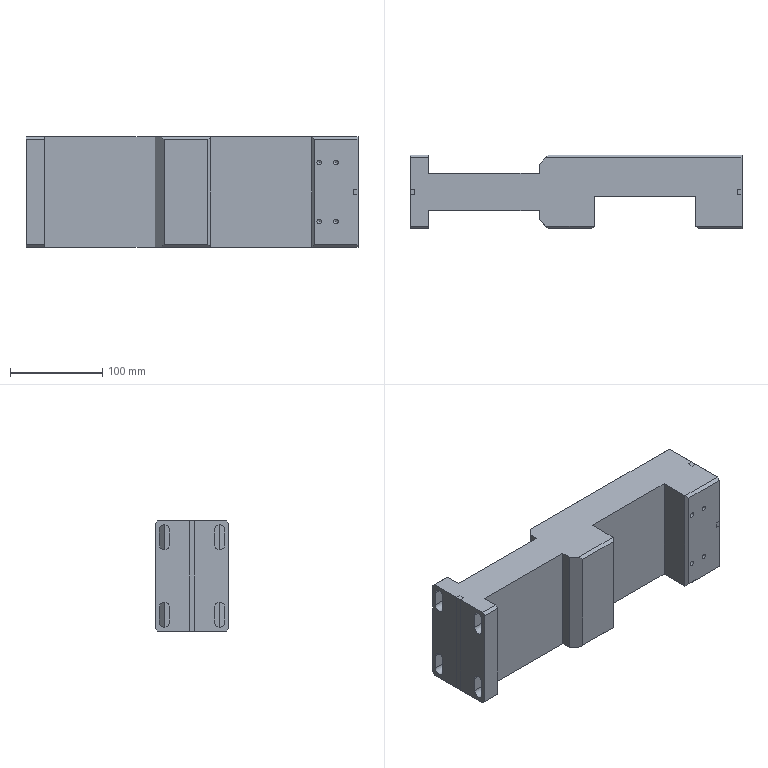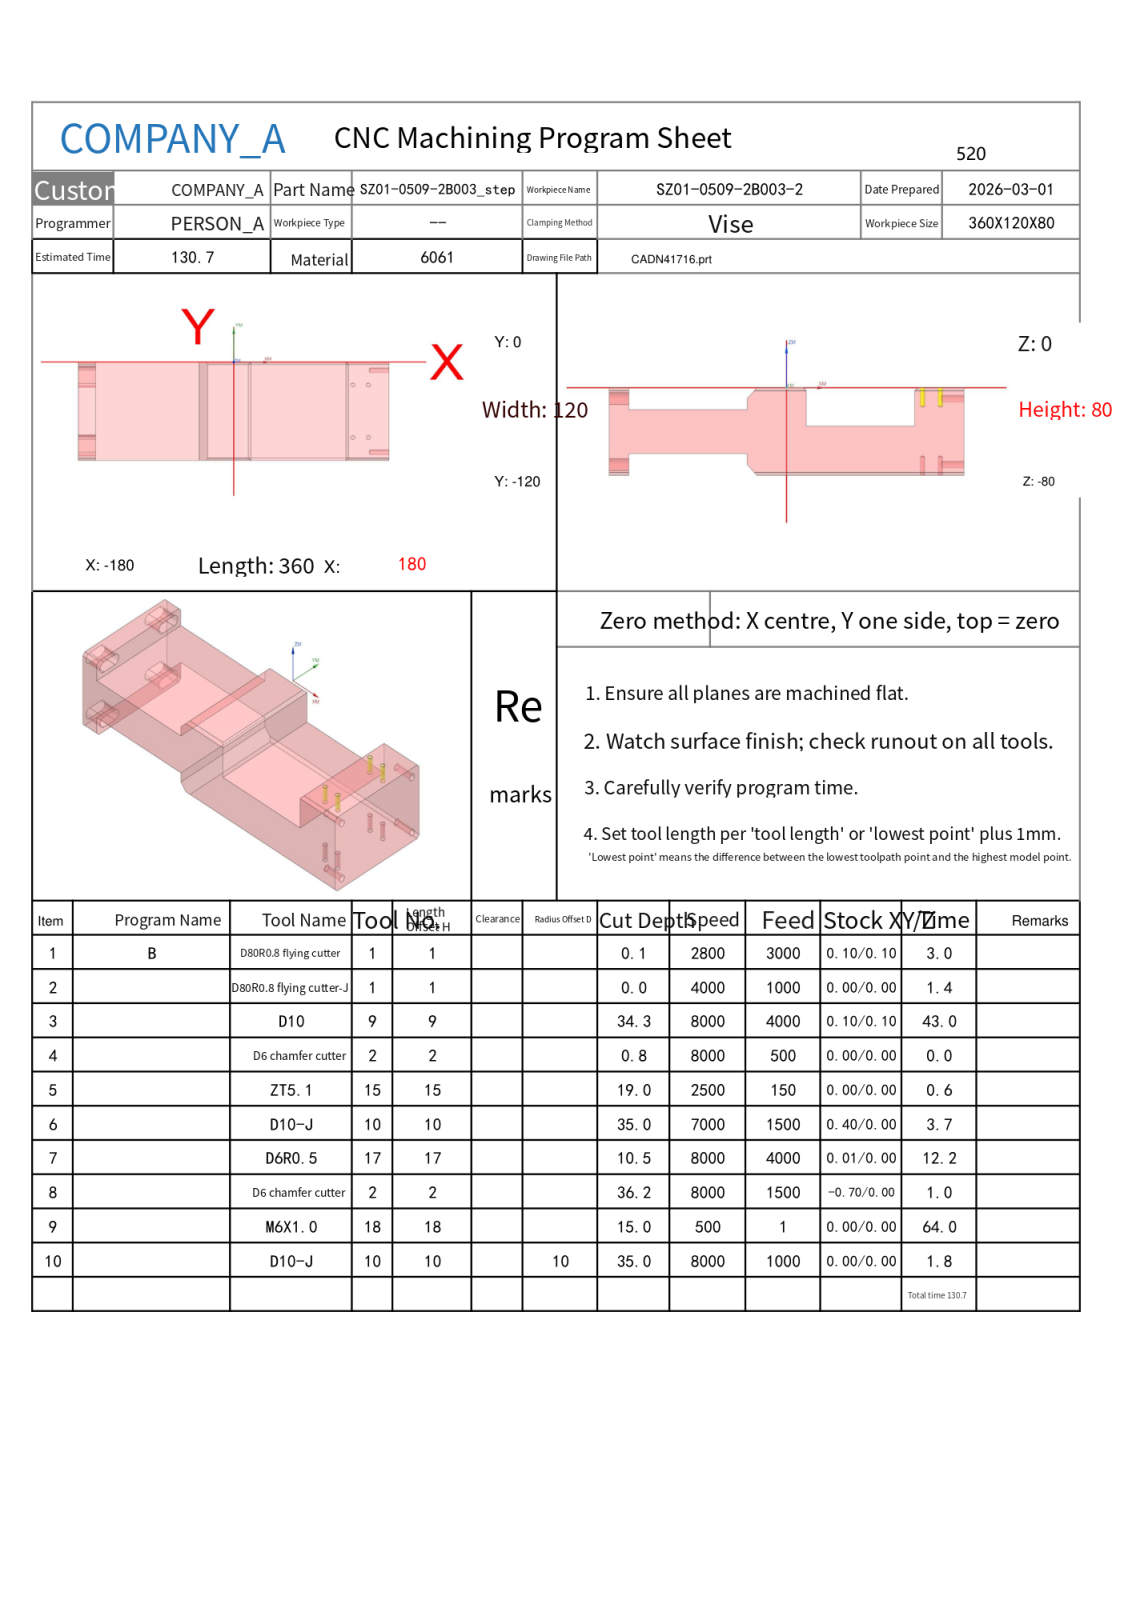NC program | NX | posted by the shop | part box 360 x 80 x 120 mm
Lines 151 to 1270 of 12457:
N3 T09 M06
(D10  D=10. R=0. H=09 ce=0.10 di=0.10)
G00 G90 G54 X-85.526 Y-134.5 M03 S8000
G43 H09 Z14.5
M08
Z.514
G01 Z-.686 F4000.
Y-127.081
G03 X-92.526 Y-120.081 I-7. J0.0
G01 X-153.947 Y-120.08
X-154.822
G02 X-155.408 Y-122.316 I-5.247 J.18
X-155.832 Y-123. I-4.662 J2.416
G01 X-156.212
G02 X-160. Y-124.228 I-3.808 J5.293
G01 X-179.919
Y-123.
X-180.
Y-124.228
Y-123.
X-180.08
X-180.079 Y-122.828
X-180.001
X-180.
X-179.999
X-179.919
X-178.519
X-160.
G03 X-154.903 Y-117.896 I-.021 J5.121
G01 X-154.866 Y-117.691
X-154.82 Y-116.969
Y-116.774
Y-116.578
Y-116.189
Y-115.297
Y-114.405
X-154.821 Y-113.513
Y-58.662
Y-3.812
X-154.822 Y-2.914
X-154.867 Y-2.301
X-154.903 Y-2.104
G03 X-160. Y2.828 I-5.117 J-.189
G01 X-178.52
X-179.92
X-179.999
X-180.
X-180.001
X-180.08
Y3.
X-180.
Y4.228
Y3.
X-179.92
Y4.228
X-159.994
G02 X-156.213 Y3. I-.026 J-6.521
G01 X-155.849
G02 X-155.456 Y2.363 I-4.505 J-3.224
X-154.823 Y.08 I-4.899 J-2.587
G01 X-44.966
X-38.144
X-38.087 Y.66
G02 X-37.123 Y3. I5.19 J-.768
G01 X-34.549
G02 X-30.757 Y4.228 I3.792 J-5.243
G01 X17.757
G02 X21.549 Y3. I0.0 J-6.471
G01 X24.114
G02 X25.148 Y.08 I-4.246 J-3.147
G01 X25.932
X124.296
X124.852
G02 X125.852 Y3. I5.632 J-.298
G01 X128.451
G02 X132.243 Y4.228 I3.792 J-5.243
G01 X179.92
Y3.
X180.
Y4.228
Y3.
X180.08
Y2.828
X180.001
X180.
X179.999
X179.92
X178.52
X132.243
G03 X127.172 Y-2.243 I0.0 J-5.071
G01 Y-117.757
G03 X132.243 Y-122.828 I5.071 J0.0
G01 X178.519
X179.919
X180.079
Y-123.
X179.919
Y-124.228
X132.243
G02 X128.452 Y-123. I0.0 J6.471
G01 X125.892
G02 X124.852 Y-120.08 I4.35 J3.193
G01 X28.427
G02 X27.486 Y-119.417 I.001 J1.
G01 X25.406 Y-113.592
G03 X24.846 Y-113.005 I-.941 J-.337
G02 X24.228 Y-112.085 I.381 J.924
G01 Y-7.915
G02 X25.223 Y-6.92 I1. J-.005
G01 X25.933
X119.177
G02 X120.172 Y-7.915 I-.005 J-1.
G01 Y-112.085
G02 X119.177 Y-113.08 I-1. J.005
G01 X28.721
G02 X28.022 Y-112.38 I.001 J.7
X28.064 Y-112.142 I.7 J0.0
G01 X31.168 Y-103.596
G03 X31.228 Y-103.256 I-.94 J.341
G01 Y-14.915
G02 X32.223 Y-13.92 I1. J-.005
G01 X112.177
G02 X113.172 Y-14.915 I-.005 J-1.
G01 Y-105.085
G02 X112.177 Y-106.08 I-1. J.005
G01 X34.923
G02 X34.323 Y-105.48 I0.0 J.6
X34.373 Y-105.241 I.6 J0.0
G01 X38.145 Y-96.562
G03 X38.228 Y-96.164 I-.917 J.398
G01 Y-21.915
G02 X39.222 Y-20.92 I1. J-.005
G01 X105.178
G02 X106.172 Y-21.915 I-.005 J-1.
G01 Y-98.085
G02 X105.178 Y-99.08 I-1. J.005
G01 X41.868
G02 X41.268 Y-98.48 I0.0 J.6
X41.319 Y-98.239 I.6 J0.0
G01 X45.143 Y-89.558
G03 X45.228 Y-89.156 I-.915 J.403
G01 Y-28.915
G02 X46.222 Y-27.92 I1. J-.005
G01 X98.178
G02 X99.172 Y-28.915 I-.005 J-1.
G01 Y-91.085
G02 X98.178 Y-92.08 I-1. J.005
G01 X48.863
G02 X48.263 Y-91.48 I0.0 J.6
X48.314 Y-91.238 I.6 J0.0
G01 X52.143 Y-82.558
G03 X52.228 Y-82.155 I-.915 J.403
G01 Y-35.914
G02 X53.222 Y-34.92 I1. J-.006
G01 X91.178
G02 X92.172 Y-35.914 I-.006 J-1.
G01 Y-84.086
G02 X91.178 Y-85.08 I-1. J.006
G01 X55.862
G02 X55.263 Y-84.48 I0.0 J.6
X55.314 Y-84.238 I.6 J0.0
G01 X59.143 Y-75.558
G03 X59.228 Y-75.155 I-.915 J.403
G01 Y-42.914
G02 X60.222 Y-41.92 I1. J-.006
G01 X84.178
G02 X85.172 Y-42.914 I-.006 J-1.
G01 Y-77.086
G02 X84.178 Y-78.08 I-1. J.006
G01 X62.862
G02 X62.263 Y-77.48 I0.0 J.6
X62.314 Y-77.238 I.6 J0.0
G01 X66.143 Y-68.558
G03 X66.228 Y-68.155 I-.915 J.403
G01 Y-49.914
G02 X67.222 Y-48.92 I1. J-.006
G01 X77.178
G02 X78.172 Y-49.914 I-.006 J-1.
G01 Y-70.086
G02 X77.178 Y-71.08 I-1. J.006
G01 X69.836
G02 X69.137 Y-70.38 I0.0 J.7
G01 X69.157 Y-70.212
X70.698 Y-63.983
G03 X70.728 Y-63.744 I-.971 J.24
G01 Y-54.414
G02 X71.722 Y-53.42 I1. J-.006
G01 X72.678
G02 X73.672 Y-54.414 I-.006 J-1.
G01 Y-65.586
G02 X72.854 Y-66.563 I-1. J.006
G03 X72.472 Y-66.721 I.182 J-.983
G01 X66.597 Y-70.735
X66.455 Y-70.853
X59.521 Y-77.787
X52.521 Y-84.787
X45.521 Y-91.788
X38.526 Y-98.79
X38.523 Y-98.793
X31.59 Y-105.811
X31.549 Y-105.855
X25.443 Y-112.829
G03 X25.198 Y-113.412 I.753 J-.658
G01 X24.536 Y-122.243
G02 X24.443 Y-122.561 I-.798 J.06
G01 X24.36 Y-122.711
G02 X24.149 Y-123. I-4.603 J3.119
G01 X21.549
G02 X17.757 Y-124.228 I-3.792 J5.243
G01 X-30.757
G02 X-34.549 Y-123. I0.0 J6.471
G01 X-37.102
G02 X-38.148 Y-120.08 I4.324 J3.195
G01 X-45.168 Y-120.082
X-89.512 Y-120.081
G02 X-90.324 Y-119.663 I.001 J1.
G01 X-94.727 Y-113.5
G03 X-95.54 Y-113.081 I-.813 J-.582
G01 X-146.826 Y-113.08
G02 X-147.821 Y-112.085 I.005 J1.
G01 Y-7.915
G02 X-146.826 Y-6.92 I1. J-.005
G01 X-140.821
X-45.023
X-38.223
G02 X-37.228 Y-7.915 I-.005 J-1.
G01 Y-111.592
G03 X-36.783 Y-112.295 I.779 J.001
G01 X-36.428 Y-112.464
X-36.248 Y-112.505
G03 X-35.828 Y-112.085 I0.0 J.42
G01 Y-2.243
G02 X-30.757 Y2.828 I5.071 J0.0
G01 X17.757
G02 X22.828 Y-2.243 I0.0 J-5.071
G01 Y-117.757
G02 X17.757 Y-122.828 I-5.071 J0.0
G01 X-30.757
G02 X-35.828 Y-117.757 I0.0 J5.071
G01 Y-112.085
G03 X-36.248 Y-111.665 I-.42 J0.0
G01 X-36.428 Y-111.705
X-37.026 Y-111.989
G03 X-37.246 Y-112.273 I.172 J-.361
G02 X-38.223 Y-113.08 I-.981 J.193
G01 X-45.023
X-45.168 Y-113.082
X-89.511 Y-113.081
G02 X-90.324 Y-112.663 I.001 J1.
G01 X-94.727 Y-106.5
G03 X-95.54 Y-106.081 I-.813 J-.582
G01 X-139.827 Y-106.08
G02 X-140.821 Y-105.085 I.005 J1.
G01 Y-14.915
G02 X-139.826 Y-13.92 I1. J-.005
G01 X-45.223
G02 X-44.228 Y-14.915 I-.005 J-1.
G01 Y-105.087
G02 X-45.225 Y-106.082 I-1. J.005
G01 X-89.511 Y-106.081
G02 X-90.324 Y-105.663 I.001 J1.
G01 X-94.726 Y-99.5
G03 X-95.539 Y-99.081 I-.813 J-.582
G01 X-132.827 Y-99.08
G02 X-133.821 Y-98.086 I.005 J1.
G01 Y-21.915
G02 X-132.827 Y-20.92 I1. J-.005
G01 X-52.222
G02 X-51.228 Y-21.915 I-.005 J-1.
G01 Y-98.087
G02 X-52.222 Y-99.082 I-1. J.005
G01 X-89.511 Y-99.081
G02 X-90.324 Y-98.663 I.001 J1.
G01 X-94.726 Y-92.5
G03 X-95.539 Y-92.081 I-.813 J-.582
G01 X-125.827
G02 X-126.821 Y-91.086 I.005 J1.
G01 Y-28.915
G02 X-125.827 Y-27.92 I1. J-.005
G01 X-59.222
G02 X-58.228 Y-28.915 I-.005 J-1.
G01 Y-91.087
G02 X-59.222 Y-92.082 I-1. J.005
G01 X-89.511 Y-92.081
G02 X-90.324 Y-91.663 I0.0 J1.
G01 X-94.726 Y-85.5
G03 X-95.539 Y-85.081 I-.814 J-.582
G01 X-118.827
G02 X-119.821 Y-84.086 I.006 J1.
G01 Y-35.914
G02 X-118.827 Y-34.92 I1. J-.006
G01 X-66.222
G02 X-65.228 Y-35.914 I-.006 J-1.
G01 Y-84.087
G02 X-66.222 Y-85.082 I-1. J.006
G01 X-89.511 Y-85.081
G02 X-90.324 Y-84.663 I0.0 J1.
G01 X-94.726 Y-78.5
G03 X-95.539 Y-78.081 I-.814 J-.582
G01 X-111.827
G02 X-112.821 Y-77.087 I.006 J1.
G01 Y-42.914
G02 X-111.827 Y-41.92 I1. J-.006
G01 X-73.222
G02 X-72.228 Y-42.914 I-.006 J-1.
G01 Y-77.087
G02 X-73.222 Y-78.082 I-1. J.006
G01 X-89.511 Y-78.081
G02 X-90.324 Y-77.663 I0.0 J1.
G01 X-94.726 Y-71.5
G03 X-95.539 Y-71.081 I-.814 J-.582
G01 X-104.827
G02 X-105.821 Y-70.087 I.006 J1.
G01 Y-49.914
G02 X-104.827 Y-48.92 I1. J-.006
G01 X-80.222
G02 X-79.228 Y-49.914 I-.006 J-1.
G01 Y-70.087
G02 X-80.222 Y-71.082 I-1. J.006
G01 X-89.51 Y-71.081
G02 X-90.324 Y-70.663 I0.0 J1.
G01 X-94.726 Y-64.5
G03 X-95.539 Y-64.081 I-.814 J-.581
G01 X-97.827
G02 X-98.821 Y-63.087 I.006 J1.
G01 Y-56.914
G02 X-97.827 Y-55.92 I1. J-.006
G01 X-87.222
G02 X-86.228 Y-56.914 I-.006 J-1.
G01 Y-63.087
G02 X-87.222 Y-64.081 I-1. J.006
G01 X-92.525
X-93.025
G03 X-100.025 Y-71.081 I0.0 J-7.
G01 Z.514
G00 Z3.
G01 X-85.526 Y-134.5 F6000.
G00 Z-.172
G01 Z-1.372 F4000.
Y-127.081
G03 X-92.526 Y-120.081 I-7. J0.0
G01 X-154.822 Y-120.08
G02 X-160.065 Y-125.151 I-5.247 J.18
G01 X-180.
X-180.085 Y-125.156
X-180.08 Y-125.071
Y-123.514
X-180.
X-179.92
X-160.
G03 X-154.9 Y-118.372 I-.053 J5.153
G01 Y-117.877
X-154.866 Y-117.691
X-154.82 Y-116.969
Y-116.774
Y-116.579
Y-116.189
Y-115.297
Y-114.405
X-154.821 Y-113.513
Y-3.812
X-154.822 Y-2.914
X-154.867 Y-2.301
X-154.9 Y-2.123
Y-1.628
G03 X-160. Y3.514 I-5.153 J-.012
G01 X-179.92
X-180.08
Y5.071
X-180.085 Y5.156
X-180. Y5.151
X-160.064
G02 X-157.129 Y4.28 I-.077 J-5.644
X-154.823 Y.08 I-3.226 J-4.504
G01 X-146.825
X-44.966
X-38.144
X-38.087 Y.66
G02 X-33.086 Y5.134 I5.19 J-.768
G01 X19.678 Y5.151
X20.578 Y5.091
G02 X25.148 Y.08 I-.71 J-5.237
G01 X25.932
X124.296
X124.852
G02 X126.141 Y3.379 I5.632 J-.298
X130.319 Y5.156 I4.179 J-4.026
X130.557 Y5.151 I0.0 J-5.803
G01 X180.
X180.085 Y5.156
X180.08 Y5.071
Y3.514
X179.92
X131.557
G03 X126.486 Y-1.557 I0.0 J-5.071
G01 Y-118.443
G03 X131.557 Y-123.514 I5.071 J0.0
G01 X179.919
X180.079
Y-124.215
X180.08 Y-125.071
X180.085 Y-125.156
X180. Y-125.151
X130.553
X129.648 Y-125.116
X128.74 Y-124.96
X127.837 Y-124.638
G02 X124.852 Y-120.08 I2.405 J4.831
G01 X29.114
G02 X28.173 Y-119.417 I.001 J1.
G01 X26.093 Y-113.592
G03 X25.533 Y-113.005 I-.941 J-.337
G02 X24.914 Y-112.084 I.381 J.925
G01 Y-7.916
G02 X25.91 Y-6.92 I1. J-.004
G01 X118.49
G02 X119.486 Y-7.916 I-.004 J-1.
G01 Y-112.084
G02 X118.49 Y-113.08 I-1. J.004
G01 X29.408
G02 X28.709 Y-112.38 I.001 J.7
X28.751 Y-112.142 I.7 J0.0
G01 X31.854 Y-103.596
G03 X31.914 Y-103.257 I-.94 J.341
G01 Y-14.916
G02 X32.91 Y-13.92 I1. J-.004
G01 X111.49
G02 X112.486 Y-14.916 I-.004 J-1.
G01 Y-105.084
G02 X111.49 Y-106.08 I-1. J.004
G01 X35.609
G02 X35.01 Y-105.48 I0.0 J.6
X35.059 Y-105.241 I.6 J0.0
G01 X38.831 Y-96.562
G03 X38.914 Y-96.164 I-.917 J.398
G01 Y-21.915
G02 X39.909 Y-20.92 I1. J-.005
G01 X104.491
G02 X105.486 Y-21.915 I-.005 J-1.
G01 Y-98.085
G02 X104.491 Y-99.08 I-1. J.005
G01 X42.554
G02 X41.954 Y-98.48 I0.0 J.6
X42.005 Y-98.239 I.6 J0.0
G01 X45.829 Y-89.558
G03 X45.914 Y-89.156 I-.915 J.403
G01 Y-28.915
G02 X46.909 Y-27.92 I1. J-.005
G01 X97.491
G02 X98.486 Y-28.915 I-.005 J-1.
G01 Y-91.085
G02 X97.491 Y-92.08 I-1. J.005
G01 X49.549
G02 X48.949 Y-91.48 I0.0 J.6
X49. Y-91.238 I.6 J0.0
G01 X52.829 Y-82.558
G03 X52.914 Y-82.155 I-.915 J.403
G01 Y-35.915
G02 X53.909 Y-34.92 I1. J-.005
G01 X90.491
G02 X91.486 Y-35.915 I-.005 J-1.
G01 Y-84.085
G02 X90.491 Y-85.08 I-1. J.005
G01 X56.549
G02 X55.949 Y-84.48 I0.0 J.6
X56. Y-84.238 I.6 J0.0
G01 X59.829 Y-75.558
G03 X59.914 Y-75.155 I-.915 J.403
G01 Y-42.915
G02 X60.909 Y-41.92 I1. J-.005
G01 X83.491
G02 X84.486 Y-42.915 I-.005 J-1.
G01 Y-77.085
G02 X83.491 Y-78.08 I-1. J.005
G01 X63.549
G02 X62.949 Y-77.48 I0.0 J.6
X63. Y-77.238 I.6 J0.0
G01 X66.829 Y-68.558
G03 X66.914 Y-68.155 I-.915 J.403
G01 Y-49.915
G02 X67.909 Y-48.92 I1. J-.005
G01 X76.491
G02 X77.486 Y-49.915 I-.005 J-1.
G01 Y-70.085
G02 X76.491 Y-71.08 I-1. J.005
G01 X70.524
G02 X69.825 Y-70.38 I0.0 J.7
G01 X69.846 Y-70.211
X71.384 Y-64.049
G03 X71.414 Y-63.807 I-.97 J.242
G01 Y-54.116
G02 X72.11 Y-53.42 I.7 J-.004
G01 X72.29
G02 X72.986 Y-54.116 I-.004 J-.7
G01 Y-65.884
G02 X72.464 Y-66.557 I-.7 J.004
G03 X72.081 Y-66.754 I.254 J-.967
G01 X67.243 Y-70.758
X67.174 Y-70.82
X60.207 Y-77.787
X53.207 Y-84.787
X46.207 Y-91.788
X39.213 Y-98.79
X39.209 Y-98.793
X32.276 Y-105.811
X32.236 Y-105.855
X26.11 Y-112.851
G03 X25.871 Y-113.382 I.753 J-.658
G01 X24.81 Y-121.66
G02 X24.751 Y-121.894 I-.992 J.128
X24.36 Y-122.711 I-5.579 J2.172
X19.757 Y-125.151 I-4.603 J3.119
G01 X19.672
X-33.096 Y-125.134
X-34.004 Y-125.019
X-34.906 Y-124.742
G02 X-38.148 Y-120.08 I2.128 J4.937
G01 X-38.91
X-45.168 Y-120.082
X-89.512 Y-120.081
G02 X-90.324 Y-119.663 I.001 J1.
G01 X-94.727 Y-113.5
G03 X-95.54 Y-113.081 I-.813 J-.582
G01 X-146.825 Y-113.08
G02 X-147.821 Y-112.084 I.004 J1.
G01 Y-7.916
G02 X-146.825 Y-6.92 I1. J-.004
G01 X-140.821
X-44.914
X-38.91
G02 X-37.914 Y-7.916 I-.004 J-1.
G01 Y-111.592
G03 X-37.469 Y-112.295 I.779 J.001
G01 X-37.114 Y-112.463
X-36.934 Y-112.504
G03 X-36.514 Y-112.084 I0.0 J.42
G01 Y-1.557
G02 X-31.443 Y3.514 I5.071 J0.0
G01 X18.443
G02 X23.514 Y-1.557 I0.0 J-5.071
G01 Y-118.443
G02 X18.443 Y-123.514 I-5.071 J0.0
G01 X-31.443
G02 X-36.514 Y-118.443 I0.0 J5.071
G01 Y-112.084
G03 X-36.934 Y-111.664 I-.42 J0.0
G01 X-37.114 Y-111.704
X-37.712 Y-111.988
G03 X-37.932 Y-112.272 I.172 J-.361
G02 X-38.91 Y-113.08 I-.981 J.192
G01 X-45.023
X-45.168 Y-113.082
X-89.511 Y-113.081
G02 X-90.324 Y-112.663 I.001 J1.
G01 X-94.727 Y-106.5
G03 X-95.54 Y-106.081 I-.813 J-.582
G01 X-139.826 Y-106.08
G02 X-140.821 Y-105.085 I.004 J1.
G01 Y-14.916
G02 X-139.826 Y-13.92 I1. J-.004
G01 X-45.91
G02 X-44.914 Y-14.916 I-.004 J-1.
G01 Y-105.087
G02 X-45.91 Y-106.082 I-1. J.004
G01 X-89.511 Y-106.081
G02 X-90.324 Y-105.663 I.001 J1.
G01 X-94.726 Y-99.5
G03 X-95.539 Y-99.081 I-.813 J-.582
G01 X-132.826 Y-99.08
G02 X-133.821 Y-98.085 I.005 J1.
G01 Y-21.915
G02 X-132.826 Y-20.92 I1. J-.005
G01 X-52.909
G02 X-51.914 Y-21.915 I-.005 J-1.
G01 Y-98.087
G02 X-52.909 Y-99.082 I-1. J.005
G01 X-89.511 Y-99.081
G02 X-90.324 Y-98.663 I.001 J1.
G01 X-94.726 Y-92.5
G03 X-95.539 Y-92.081 I-.813 J-.582
G01 X-125.826
G02 X-126.821 Y-91.085 I.005 J1.
G01 Y-28.915
G02 X-125.826 Y-27.92 I1. J-.005
G01 X-59.909
G02 X-58.914 Y-28.915 I-.005 J-1.
G01 Y-91.087
G02 X-59.909 Y-92.082 I-1. J.005
G01 X-89.511 Y-92.081
G02 X-90.324 Y-91.663 I0.0 J1.
G01 X-94.726 Y-85.5
G03 X-95.539 Y-85.081 I-.814 J-.582
G01 X-118.826
G02 X-119.821 Y-84.086 I.005 J1.
G01 Y-35.915
G02 X-118.826 Y-34.92 I1. J-.005
G01 X-66.909
G02 X-65.914 Y-35.915 I-.005 J-1.
G01 Y-84.087
G02 X-66.909 Y-85.082 I-1. J.005
G01 X-89.511 Y-85.081
G02 X-90.324 Y-84.663 I0.0 J1.
G01 X-94.726 Y-78.5
G03 X-95.539 Y-78.081 I-.814 J-.582
G01 X-111.826
G02 X-112.821 Y-77.086 I.005 J1.
G01 Y-42.915
G02 X-111.826 Y-41.92 I1. J-.005
G01 X-73.909
G02 X-72.914 Y-42.915 I-.005 J-1.
G01 Y-77.087
G02 X-73.909 Y-78.082 I-1. J.005
G01 X-89.511 Y-78.081
G02 X-90.324 Y-77.663 I0.0 J1.
G01 X-94.726 Y-71.5
G03 X-95.539 Y-71.081 I-.814 J-.582
G01 X-104.827
G02 X-105.821 Y-70.086 I.005 J1.
G01 Y-49.915
G02 X-104.826 Y-48.92 I1. J-.005
G01 X-80.909
G02 X-79.914 Y-49.915 I-.005 J-1.
G01 Y-70.087
G02 X-80.909 Y-71.082 I-1. J.005
G01 X-89.51 Y-71.081
G02 X-90.324 Y-70.663 I0.0 J1.
G01 X-94.726 Y-64.5
G03 X-95.539 Y-64.081 I-.814 J-.581
G01 X-97.827
G02 X-98.821 Y-63.086 I.005 J1.
G01 Y-56.915
G02 X-97.827 Y-55.92 I1. J-.005
G01 X-87.909
G02 X-86.914 Y-56.915 I-.005 J-1.
G01 Y-63.087
G02 X-87.909 Y-64.081 I-1. J.005
G01 X-92.525
X-93.025
G03 X-100.025 Y-71.081 I0.0 J-7.
G01 Z-.172
G00 Z3.
G01 X-85.526 Y-134.5 F6000.
G00 Z-.859
G01 Z-2.059 F4000.
Y-127.081
G03 X-92.526 Y-120.081 I-7. J0.0
G01 X-154.822 Y-120.08
G02 X-160.065 Y-125.151 I-5.247 J.18
G01 X-180.
X-180.085 Y-125.156
X-180.08 Y-125.071
Y-124.2
X-180.
X-179.92
X-160.
G03 X-154.9 Y-119.059 I-.052 J5.152
G01 Y-117.877
X-154.866 Y-117.691
X-154.82 Y-116.969
Y-116.774
Y-116.579
Y-116.189
Y-115.297
Y-114.405
X-154.821 Y-113.513
Y-3.812
X-154.822 Y-2.914
X-154.867 Y-2.301
X-154.9 Y-2.123
Y-.941
G03 X-160. Y4.2 I-5.152 J-.01
G01 X-179.92
X-180.08
Y5.071
X-180.085 Y5.156
X-180. Y5.151
X-160.064
G02 X-157.129 Y4.28 I-.077 J-5.644
X-154.823 Y.08 I-3.226 J-4.504
G01 X-146.826
X-44.966
X-38.144
X-38.087 Y.66
G02 X-33.086 Y5.134 I5.19 J-.768
G01 X19.678 Y5.151
X20.578 Y5.091
G02 X25.148 Y.08 I-.71 J-5.237
G01 X25.932
X124.296
X124.852
G02 X126.141 Y3.379 I5.632 J-.298
X130.319 Y5.156 I4.179 J-4.026
X130.557 Y5.151 I0.0 J-5.803
G01 X180.
X180.085 Y5.156
X180.08 Y5.071
Y4.2
X179.92
X130.871
G03 X125.8 Y-.871 I0.0 J-5.071
G01 Y-119.129
G03 X130.871 Y-124.2 I5.071 J0.0
G01 X179.919
X180.079
X180.08 Y-125.071
X180.085 Y-125.156
X180. Y-125.151
X130.553
X129.648 Y-125.116
X128.74 Y-124.96
X127.837 Y-124.638
G02 X124.852 Y-120.08 I2.405 J4.831
G01 X29.8
G02 X28.859 Y-119.417 I.001 J1.
G01 X26.779 Y-113.592
G03 X26.219 Y-113.005 I-.941 J-.337
G02 X25.6 Y-112.084 I.381 J.925
G01 Y-7.916
G02 X26.596 Y-6.92 I1. J-.004
G01 X117.804
G02 X118.8 Y-7.916 I-.004 J-1.
G01 Y-112.084
G02 X117.804 Y-113.08 I-1. J.004
G01 X30.094
G02 X29.395 Y-112.38 I.001 J.7
X29.437 Y-112.142 I.7 J0.0
G01 X32.54 Y-103.596
G03 X32.6 Y-103.257 I-.94 J.341
G01 Y-14.915
G02 X33.595 Y-13.92 I1. J-.005
G01 X110.805
G02 X111.8 Y-14.915 I-.005 J-1.
G01 Y-105.085
G02 X110.805 Y-106.08 I-1. J.005
G01 X36.295
G02 X35.696 Y-105.48 I0.0 J.6
X35.745 Y-105.241 I.6 J0.0
G01 X39.517 Y-96.562
G03 X39.6 Y-96.164 I-.917 J.398
G01 Y-21.915
G02 X40.595 Y-20.92 I1. J-.005
G01 X103.805
G02 X104.8 Y-21.915 I-.005 J-1.
G01 Y-98.085
G02 X103.805 Y-99.08 I-1. J.005
G01 X43.24
G02 X42.641 Y-98.48 I0.0 J.6
X42.691 Y-98.239 I.6 J0.0
G01 X46.515 Y-89.558
G03 X46.6 Y-89.156 I-.915 J.403
G01 Y-28.915
G02 X47.595 Y-27.92 I1. J-.005
G01 X96.805
G02 X97.8 Y-28.915 I-.005 J-1.
G01 Y-91.085
G02 X96.805 Y-92.08 I-1. J.005
G01 X50.235
G02 X49.636 Y-91.48 I0.0 J.6
X49.686 Y-91.238 I.6 J0.0
G01 X53.515 Y-82.558
G03 X53.6 Y-82.155 I-.915 J.403
G01 Y-35.915
G02 X54.595 Y-34.92 I1. J-.005
G01 X89.805
G02 X90.8 Y-35.915 I-.005 J-1.
G01 Y-84.085
G02 X89.805 Y-85.08 I-1. J.005
G01 X57.235
G02 X56.635 Y-84.48 I0.0 J.6
X56.686 Y-84.238 I.6 J0.0
G01 X60.515 Y-75.558
G03 X60.6 Y-75.155 I-.915 J.403
G01 Y-42.915
G02 X61.595 Y-41.92 I1. J-.005
G01 X82.805
G02 X83.8 Y-42.915 I-.005 J-1.
G01 Y-77.085
G02 X82.805 Y-78.08 I-1. J.005
G01 X64.235
G02 X63.635 Y-77.48 I0.0 J.6
X63.686 Y-77.238 I.6 J0.0
G01 X67.515 Y-68.558
G03 X67.6 Y-68.155 I-.915 J.403
G01 Y-49.915
G02 X68.595 Y-48.92 I1. J-.005
G01 X75.805
G02 X76.8 Y-49.915 I-.005 J-1.
G01 Y-70.085
G02 X75.805 Y-71.08 I-1. J.005
G01 X70.634
G03 X70.055 Y-71.265 I.001 J-1.
G01 X60.961 Y-77.739
X60.834 Y-77.846
X53.893 Y-84.787
X46.893 Y-91.788
X39.899 Y-98.79
X39.896 Y-98.793
X32.962 Y-105.811
X32.922 Y-105.855
X26.772 Y-112.879
G03 X26.544 Y-113.342 I.753 J-.658
G01 X24.997 Y-121.1
X24.988 Y-121.14
G02 X24.36 Y-122.711 I-5.817 J1.417
X19.757 Y-125.151 I-4.603 J3.119
G01 X19.672
X-33.096 Y-125.134
X-34.004 Y-125.019
X-34.906 Y-124.742
G02 X-38.148 Y-120.08 I2.128 J4.937
G01 X-39.596
X-45.168 Y-120.082
X-89.512 Y-120.081
G02 X-90.324 Y-119.663 I.001 J1.
G01 X-94.727 Y-113.5
G03 X-95.54 Y-113.081 I-.813 J-.582
G01 X-146.826 Y-113.08
G02 X-147.821 Y-112.084 I.004 J1.
G01 Y-7.916
G02 X-146.826 Y-6.92 I1. J-.004
G01 X-45.023
X-39.596
G02 X-38.6 Y-7.916 I-.004 J-1.
G01 Y-111.592
G03 X-38.155 Y-112.295 I.779 J.001
G01 X-37.8 Y-112.464
X-37.62 Y-112.504
G03 X-37.2 Y-112.084 I0.0 J.42
G01 Y-.871
G02 X-32.129 Y4.2 I5.071 J0.0
G01 X19.129
G02 X24.2 Y-.871 I0.0 J-5.071
G01 Y-119.129
G02 X19.129 Y-124.2 I-5.071 J0.0
G01 X-32.129
G02 X-37.2 Y-119.129 I0.0 J5.071
G01 Y-112.084
G03 X-37.62 Y-111.664 I-.42 J0.0
G01 X-37.8 Y-111.705
X-38.398 Y-111.988
G03 X-38.619 Y-112.272 I.172 J-.361
G02 X-39.596 Y-113.08 I-.981 J.192
G01 X-45.023
X-45.168 Y-113.082
X-89.511 Y-113.081
G02 X-90.324 Y-112.663 I.001 J1.
G01 X-94.727 Y-106.5
G03 X-95.54 Y-106.081 I-.813 J-.582
G01 X-139.826 Y-106.08
G02 X-140.821 Y-105.085 I.005 J1.
G01 Y-14.915
G02 X-139.826 Y-13.92 I1. J-.005
G01 X-46.595
G02 X-45.6 Y-14.915 I-.005 J-1.
G01 Y-105.087
G02 X-46.595 Y-106.082 I-1. J.005
G01 X-89.511 Y-106.081
G02 X-90.324 Y-105.663 I.001 J1.
G01 X-94.726 Y-99.5
G03 X-95.539 Y-99.081 I-.813 J-.582
G01 X-132.826 Y-99.08
G02 X-133.821 Y-98.085 I.005 J1.
G01 Y-21.915
G02 X-132.826 Y-20.92 I1. J-.005
G01 X-53.595
G02 X-52.6 Y-21.915 I-.005 J-1.
G01 Y-98.087
G02 X-53.595 Y-99.082 I-1. J.005
G01 X-89.511 Y-99.081
G02 X-90.324 Y-98.663 I.001 J1.
G01 X-94.726 Y-92.5
G03 X-95.539 Y-92.081 I-.813 J-.582
G01 X-125.826
G02 X-126.821 Y-91.086 I.005 J1.
G01 Y-28.915
G02 X-125.826 Y-27.92 I1. J-.005
G01 X-60.595
G02 X-59.6 Y-28.915 I-.005 J-1.
G01 Y-91.087
G02 X-60.595 Y-92.082 I-1. J.005
G01 X-89.511 Y-92.081
G02 X-90.324 Y-91.663 I0.0 J1.
G01 X-94.726 Y-85.5
G03 X-95.539 Y-85.081 I-.813 J-.582
G01 X-118.827
G02 X-119.821 Y-84.086 I.005 J1.
G01 Y-35.915
G02 X-118.827 Y-34.92 I1. J-.005
G01 X-67.595
G02 X-66.6 Y-35.915 I-.005 J-1.
G01 Y-84.087
G02 X-67.595 Y-85.082 I-1. J.005
G01 X-89.511 Y-85.081
G02 X-90.324 Y-84.663 I0.0 J1.
G01 X-94.726 Y-78.5
G03 X-95.539 Y-78.081 I-.814 J-.582
G01 X-111.827
G02 X-112.821 Y-77.086 I.005 J1.
G01 Y-42.915
G02 X-111.827 Y-41.92 I1. J-.005
G01 X-74.595
G02 X-73.6 Y-42.915 I-.005 J-1.
G01 Y-77.087
G02 X-74.595 Y-78.082 I-1. J.005
G01 X-89.511 Y-78.081
G02 X-90.324 Y-77.663 I0.0 J1.
G01 X-94.726 Y-71.5
G03 X-95.539 Y-71.081 I-.814 J-.581
G01 X-104.827
G02 X-105.821 Y-70.086 I.005 J1.
G01 Y-49.915
G02 X-104.827 Y-48.92 I1. J-.005
G01 X-81.595
G02 X-80.6 Y-49.915 I-.005 J-1.
G01 Y-70.087
G02 X-81.595 Y-71.082 I-1. J.005
G01 X-89.51 Y-71.081
G02 X-90.324 Y-70.663 I0.0 J1.
G01 X-94.726 Y-64.5
G03 X-95.539 Y-64.081 I-.814 J-.581
G01 X-97.827
G02 X-98.821 Y-63.087 I.005 J1.
G01 Y-56.915
G02 X-97.827 Y-55.92 I1. J-.005
G01 X-88.595
G02 X-87.6 Y-56.915 I-.005 J-1.
G01 Y-63.087
G02 X-88.595 Y-64.081 I-1. J.005
G01 X-92.525
X-93.025
G03 X-100.025 Y-71.081 I0.0 J-7.
G01 Z-.859
G00 Z3.
G01 X-85.526 Y-134.5 F6000.
G00 Z-1.545
G01 Z-2.745 F4000.
Y-127.081
G03 X-92.526 Y-120.081 I-7. J0.0
G01 X-154.822 Y-120.08
G02 X-160.065 Y-125.151 I-5.247 J.18
G01 X-180.
X-180.085 Y-125.156
X-180.08 Y-125.071
Y-124.886
X-180.
X-179.999
X-179.92
X-160.
G03 X-154.9 Y-119.766 I-.021 J5.121
G01 Y-119.745
Y-117.877
X-154.866 Y-117.691
X-154.82 Y-116.969
Y-116.774
Y-116.579
Y-116.189
Y-115.297
Y-114.405
X-154.821 Y-113.513
Y-3.812
X-154.822 Y-2.914
X-154.867 Y-2.301
X-154.9 Y-2.123
Y-.255
Y-.234
G03 X-160. Y4.886 I-5.121 J0.0
G01 X-179.92
X-179.999
X-180.
X-180.08
Y5.071
X-180.085 Y5.156
X-180. Y5.151
X-160.064
G02 X-157.129 Y4.28 I-.077 J-5.644
X-154.823 Y.08 I-3.226 J-4.504
G01 X-146.826
X-44.966
X-38.144
X-38.087 Y.66
G02 X-33.086 Y5.134 I5.19 J-.768
G01 X19.678 Y5.151
X20.578 Y5.091
G02 X25.148 Y.08 I-.71 J-5.237
G01 X25.932
X124.296
X124.852
G02 X126.141 Y3.379 I5.632 J-.298
X130.319 Y5.156 I4.179 J-4.026
X130.557 Y5.151 I0.0 J-5.803
G01 X180.
X180.085 Y5.156
X180.08 Y5.071
Y4.886
X180.
X179.999
X179.92
X130.184
G03 X125.114 Y-.184 I0.0 J-5.071
G01 Y-119.816
G03 X130.184 Y-124.886 I5.071 J0.0
G01 X179.92
X180.08
Y-125.071
X180.085 Y-125.156
X180. Y-125.151
X130.553
X129.648 Y-125.116
X128.74 Y-124.96
X127.837 Y-124.638
G02 X124.852 Y-120.08 I2.405 J4.831
G01 X30.486
G02 X29.545 Y-119.417 I.001 J1.
G01 X27.464 Y-113.592
G03 X26.905 Y-113.005 I-.941 J-.337
G02 X26.286 Y-112.085 I.381 J.924
G01 Y-7.915
G02 X27.282 Y-6.92 I1. J-.005
G01 X117.118
G02 X118.114 Y-7.915 I-.005 J-1.
G01 Y-112.085
G02 X117.118 Y-113.08 I-1. J.005
G01 X30.78
G02 X30.081 Y-112.38 I.001 J.7
X30.123 Y-112.142 I.7 J0.0
G01 X33.226 Y-103.596
G03 X33.286 Y-103.256 I-.94 J.341
G01 Y-14.915
G02 X34.281 Y-13.92 I1. J-.005
G01 X110.119
G02 X111.114 Y-14.915 I-.005 J-1.
G01 Y-105.085
G02 X110.119 Y-106.08 I-1. J.005
G01 X36.982
G02 X36.382 Y-105.48 I.001 J.6
X36.432 Y-105.241 I.6 J0.0
G01 X40.204 Y-96.562
G03 X40.286 Y-96.164 I-.917 J.398
G01 Y-21.915
G02 X41.281 Y-20.92 I1. J-.005
G01 X103.119
G02 X104.114 Y-21.915 I-.005 J-1.
G01 Y-98.085
G02 X103.119 Y-99.08 I-1. J.005
G01 X43.926
G02 X43.327 Y-98.48 I0.0 J.6
X43.378 Y-98.239 I.6 J0.0
G01 X47.202 Y-89.558
G03 X47.286 Y-89.156 I-.915 J.403
G01 Y-28.915
G02 X48.281 Y-27.92 I1. J-.005
G01 X96.119
G02 X97.114 Y-28.915 I-.005 J-1.
G01 Y-91.085
G02 X96.119 Y-92.08 I-1. J.005
G01 X50.921
G02 X50.322 Y-91.48 I0.0 J.6
X50.373 Y-91.238 I.6 J0.0
G01 X54.201 Y-82.558
G03 X54.286 Y-82.155 I-.915 J.403
G01 Y-35.914
G02 X55.281 Y-34.92 I1. J-.006
G01 X89.119
G02 X90.114 Y-35.914 I-.006 J-1.
G01 Y-84.086
G02 X89.119 Y-85.08 I-1. J.006
G01 X57.921
G02 X57.321 Y-84.48 I0.0 J.6
X57.372 Y-84.238 I.6 J0.0
G01 X61.201 Y-75.558
G03 X61.286 Y-75.155 I-.915 J.403
G01 Y-42.914
G02 X62.281 Y-41.92 I1. J-.006
G01 X82.119
G02 X83.114 Y-42.914 I-.006 J-1.
G01 Y-77.086
G02 X82.119 Y-78.08 I-1. J.006
G01 X64.921
G02 X64.321 Y-77.48 I0.0 J.6
X64.372 Y-77.238 I.6 J0.0
G01 X68.201 Y-68.558
G03 X68.286 Y-68.155 I-.915 J.403
G01 Y-49.914
G02 X69.281 Y-48.92 I1. J-.006
G01 X75.119
G02 X76.114 Y-49.914 I-.006 J-1.
G01 Y-70.086
G02 X75.119 Y-71.08 I-1. J.006
G01 X71.32
G03 X70.741 Y-71.265 I.001 J-1.
G01 X61.647 Y-77.739
X61.52 Y-77.846
X54.579 Y-84.787
X47.58 Y-91.788
X40.585 Y-98.79
X40.582 Y-98.793
X33.648 Y-105.811
X33.608 Y-105.855
X27.423 Y-112.919
G03 X27.219 Y-113.285 I.753 J-.658
G01 X25.181 Y-119.972
G03 X25.14 Y-120.185 I.957 J-.291
G02 X24.36 Y-122.711 I-5.969 J.462
X19.757 Y-125.151 I-4.603 J3.119
G01 X19.672
X-33.096 Y-125.134
X-34.004 Y-125.019
X-34.906 Y-124.742
G02 X-38.148 Y-120.08 I2.128 J4.937
G01 X-40.282
X-45.168 Y-120.082
X-89.512 Y-120.081
G02 X-90.324 Y-119.663 I.001 J1.
G01 X-94.727 Y-113.5
G03 X-95.54 Y-113.081 I-.813 J-.582
G01 X-146.826 Y-113.08
G02 X-147.821 Y-112.085 I.005 J1.
G01 Y-7.915
G02 X-146.826 Y-6.92 I1. J-.005
G01 X-45.023